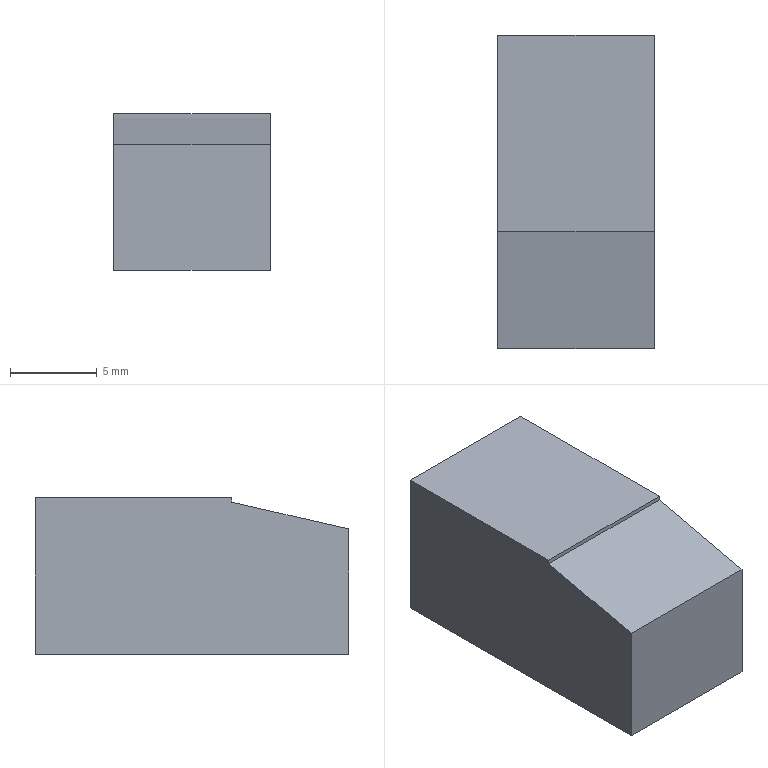Part | SolidWorks | features BaseBody 1 | 1 solid | 8 faces | box 9 x 18 x 9 mm | volume 1396 mm3 | plane 8
STEP:
#1=CARTESIAN_POINT('',(-102.,182.,178.223));
#2=VERTEX_POINT('',#1);
#3=CARTESIAN_POINT('',(-102.,188.726,179.763));
#4=VERTEX_POINT('',#3);
#5=CARTESIAN_POINT('',(-102.,199.493,182.228));
#6=DIRECTION('',(0.,0.9748,0.2232));
#7=VECTOR('',#6,1000.);
#8=LINE('',#5,#7);
#9=EDGE_CURVE('',#2,#4,#8,.T.);
#10=ORIENTED_EDGE('',*,*,#9,.T.);
#11=CARTESIAN_POINT('',(-102.,188.726,180.013));
#12=VERTEX_POINT('',#11);
#13=CARTESIAN_POINT('',(-102.,188.726,180.013));
#14=DIRECTION('',(0.,0.,1.));
#15=VECTOR('',#14,1000.);
#16=LINE('',#13,#15);
#17=EDGE_CURVE('',#4,#12,#16,.T.);
#18=ORIENTED_EDGE('',*,*,#17,.T.);
#19=CARTESIAN_POINT('',(-102.,200.,180.013));
#20=VERTEX_POINT('',#19);
#21=CARTESIAN_POINT('',(-102.,200.,180.013));
#22=DIRECTION('',(0.,-1.,0.));
#23=VECTOR('',#22,1000.);
#24=LINE('',#21,#23);
#25=EDGE_CURVE('',#20,#12,#24,.T.);
#26=ORIENTED_EDGE('',*,*,#25,.F.);
#27=CARTESIAN_POINT('',(-102.,200.,171.013));
#28=VERTEX_POINT('',#27);
#29=CARTESIAN_POINT('',(-102.,200.,180.013));
#30=DIRECTION('',(0.,0.,-1.));
#31=VECTOR('',#30,1000.);
#32=LINE('',#29,#31);
#33=EDGE_CURVE('',#20,#28,#32,.T.);
#34=ORIENTED_EDGE('',*,*,#33,.T.);
#35=CARTESIAN_POINT('',(-102.,182.,171.013));
#36=VERTEX_POINT('',#35);
#37=CARTESIAN_POINT('',(-102.,200.,171.013));
#38=DIRECTION('',(0.,-1.,0.));
#39=VECTOR('',#38,1000.);
#40=LINE('',#37,#39);
#41=EDGE_CURVE('',#28,#36,#40,.T.);
#42=ORIENTED_EDGE('',*,*,#41,.T.);
#43=CARTESIAN_POINT('',(-102.,182.,180.013));
#44=DIRECTION('',(0.,0.,-1.));
#45=VECTOR('',#44,1000.);
#46=LINE('',#43,#45);
#47=EDGE_CURVE('',#2,#36,#46,.T.);
#48=ORIENTED_EDGE('',*,*,#47,.F.);
#49=EDGE_LOOP('',(#10,#18,#26,#34,#42,#48));
#50=FACE_OUTER_BOUND('',#49,.T.);
#51=CARTESIAN_POINT('',(-102.,200.,180.013));
#52=DIRECTION('',(1.,0.,0.));
#53=DIRECTION('',(0.,0.,-1.));
#54=AXIS2_PLACEMENT_3D('',#51,#52,#53);
#55=PLANE('',#54);
#56=ADVANCED_FACE('',(#50),#55,.F.);
#57=CARTESIAN_POINT('',(-93.,182.,178.223));
#58=VERTEX_POINT('',#57);
#59=CARTESIAN_POINT('',(-93.,182.,171.013));
#60=VERTEX_POINT('',#59);
#61=CARTESIAN_POINT('',(-93.,182.,180.013));
#62=DIRECTION('',(0.,0.,-1.));
#63=VECTOR('',#62,1000.);
#64=LINE('',#61,#63);
#65=EDGE_CURVE('',#58,#60,#64,.T.);
#66=ORIENTED_EDGE('',*,*,#65,.F.);
#67=CARTESIAN_POINT('',(-71.07,182.,178.223));
#68=DIRECTION('',(-1.,0.,0.));
#69=VECTOR('',#68,1000.);
#70=LINE('',#67,#69);
#71=EDGE_CURVE('',#58,#2,#70,.T.);
#72=ORIENTED_EDGE('',*,*,#71,.T.);
#73=ORIENTED_EDGE('',*,*,#47,.T.);
#74=CARTESIAN_POINT('',(-102.,182.,171.013));
#75=DIRECTION('',(1.,0.,0.));
#76=VECTOR('',#75,1000.);
#77=LINE('',#74,#76);
#78=EDGE_CURVE('',#36,#60,#77,.T.);
#79=ORIENTED_EDGE('',*,*,#78,.T.);
#80=EDGE_LOOP('',(#66,#72,#73,#79));
#81=FACE_OUTER_BOUND('',#80,.T.);
#82=CARTESIAN_POINT('',(-102.,182.,180.013));
#83=DIRECTION('',(0.,1.,0.));
#84=DIRECTION('',(0.,0.,1.));
#85=AXIS2_PLACEMENT_3D('',#82,#83,#84);
#86=PLANE('',#85);
#87=ADVANCED_FACE('',(#81),#86,.F.);
#88=CARTESIAN_POINT('',(-93.,188.726,180.013));
#89=VERTEX_POINT('',#88);
#90=CARTESIAN_POINT('',(-93.,200.,180.013));
#91=VERTEX_POINT('',#90);
#92=CARTESIAN_POINT('',(-93.,188.,180.013));
#93=DIRECTION('',(0.,1.,0.));
#94=VECTOR('',#93,1000.);
#95=LINE('',#92,#94);
#96=EDGE_CURVE('',#89,#91,#95,.T.);
#97=ORIENTED_EDGE('',*,*,#96,.F.);
#98=CARTESIAN_POINT('',(-93.,188.726,179.763));
#99=VERTEX_POINT('',#98);
#100=CARTESIAN_POINT('',(-93.,188.726,180.013));
#101=DIRECTION('',(0.,0.,-1.));
#102=VECTOR('',#101,1000.);
#103=LINE('',#100,#102);
#104=EDGE_CURVE('',#89,#99,#103,.T.);
#105=ORIENTED_EDGE('',*,*,#104,.T.);
#106=CARTESIAN_POINT('',(-93.,188.091,179.618));
#107=DIRECTION('',(0.,-0.9748,-0.2232));
#108=VECTOR('',#107,1000.);
#109=LINE('',#106,#108);
#110=EDGE_CURVE('',#99,#58,#109,.T.);
#111=ORIENTED_EDGE('',*,*,#110,.T.);
#112=ORIENTED_EDGE('',*,*,#65,.T.);
#113=CARTESIAN_POINT('',(-93.,200.,171.013));
#114=VERTEX_POINT('',#113);
#115=CARTESIAN_POINT('',(-93.,188.,171.013));
#116=DIRECTION('',(0.,1.,0.));
#117=VECTOR('',#116,1000.);
#118=LINE('',#115,#117);
#119=EDGE_CURVE('',#60,#114,#118,.T.);
#120=ORIENTED_EDGE('',*,*,#119,.T.);
#121=CARTESIAN_POINT('',(-93.,200.,180.013));
#122=DIRECTION('',(0.,0.,-1.));
#123=VECTOR('',#122,1000.);
#124=LINE('',#121,#123);
#125=EDGE_CURVE('',#91,#114,#124,.T.);
#126=ORIENTED_EDGE('',*,*,#125,.F.);
#127=EDGE_LOOP('',(#97,#105,#111,#112,#120,#126));
#128=FACE_OUTER_BOUND('',#127,.T.);
#129=CARTESIAN_POINT('',(-93.,188.,180.013));
#130=DIRECTION('',(-1.,0.,0.));
#131=DIRECTION('',(0.,0.,1.));
#132=AXIS2_PLACEMENT_3D('',#129,#130,#131);
#133=PLANE('',#132);
#134=ADVANCED_FACE('',(#128),#133,.F.);
#135=CARTESIAN_POINT('',(-93.,200.,171.013));
#136=DIRECTION('',(-1.,0.,0.));
#137=VECTOR('',#136,1000.);
#138=LINE('',#135,#137);
#139=EDGE_CURVE('',#114,#28,#138,.T.);
#140=ORIENTED_EDGE('',*,*,#139,.T.);
#141=ORIENTED_EDGE('',*,*,#33,.F.);
#142=CARTESIAN_POINT('',(-93.,200.,180.013));
#143=DIRECTION('',(-1.,0.,0.));
#144=VECTOR('',#143,1000.);
#145=LINE('',#142,#144);
#146=EDGE_CURVE('',#91,#20,#145,.T.);
#147=ORIENTED_EDGE('',*,*,#146,.F.);
#148=ORIENTED_EDGE('',*,*,#125,.T.);
#149=EDGE_LOOP('',(#140,#141,#147,#148));
#150=FACE_OUTER_BOUND('',#149,.T.);
#151=CARTESIAN_POINT('',(-93.,200.,180.013));
#152=DIRECTION('',(0.,-1.,0.));
#153=DIRECTION('',(0.,0.,-1.));
#154=AXIS2_PLACEMENT_3D('',#151,#152,#153);
#155=PLANE('',#154);
#156=ADVANCED_FACE('',(#150),#155,.F.);
#157=CARTESIAN_POINT('',(-71.07,188.726,180.013));
#158=DIRECTION('',(-1.,0.,0.));
#159=VECTOR('',#158,1000.);
#160=LINE('',#157,#159);
#161=EDGE_CURVE('',#89,#12,#160,.T.);
#162=ORIENTED_EDGE('',*,*,#161,.F.);
#163=ORIENTED_EDGE('',*,*,#96,.T.);
#164=ORIENTED_EDGE('',*,*,#146,.T.);
#165=ORIENTED_EDGE('',*,*,#25,.T.);
#166=EDGE_LOOP('',(#162,#163,#164,#165));
#167=FACE_OUTER_BOUND('',#166,.T.);
#168=CARTESIAN_POINT('',(7.,0.,180.013));
#169=DIRECTION('',(0.,0.,1.));
#170=DIRECTION('',(1.,0.,0.));
#171=AXIS2_PLACEMENT_3D('',#168,#169,#170);
#172=PLANE('',#171);
#173=ADVANCED_FACE('',(#167),#172,.T.);
#174=ORIENTED_EDGE('',*,*,#41,.F.);
#175=ORIENTED_EDGE('',*,*,#139,.F.);
#176=ORIENTED_EDGE('',*,*,#119,.F.);
#177=ORIENTED_EDGE('',*,*,#78,.F.);
#178=EDGE_LOOP('',(#174,#175,#176,#177));
#179=FACE_OUTER_BOUND('',#178,.T.);
#180=CARTESIAN_POINT('',(7.,0.,171.013));
#181=DIRECTION('',(0.,0.,1.));
#182=DIRECTION('',(1.,0.,0.));
#183=AXIS2_PLACEMENT_3D('',#180,#181,#182);
#184=PLANE('',#183);
#185=ADVANCED_FACE('',(#179),#184,.F.);
#186=ORIENTED_EDGE('',*,*,#71,.F.);
#187=ORIENTED_EDGE('',*,*,#110,.F.);
#188=CARTESIAN_POINT('',(-71.07,188.726,179.763));
#189=DIRECTION('',(1.,0.,0.));
#190=VECTOR('',#189,1000.);
#191=LINE('',#188,#190);
#192=EDGE_CURVE('',#4,#99,#191,.T.);
#193=ORIENTED_EDGE('',*,*,#192,.F.);
#194=ORIENTED_EDGE('',*,*,#9,.F.);
#195=EDGE_LOOP('',(#186,#187,#193,#194));
#196=FACE_OUTER_BOUND('',#195,.T.);
#197=CARTESIAN_POINT('',(-71.07,188.726,179.763));
#198=DIRECTION('',(0.,0.2232,-0.9748));
#199=DIRECTION('',(0.,-0.9748,-0.2232));
#200=AXIS2_PLACEMENT_3D('',#197,#198,#199);
#201=PLANE('',#200);
#202=ADVANCED_FACE('',(#196),#201,.F.);
#203=ORIENTED_EDGE('',*,*,#192,.T.);
#204=ORIENTED_EDGE('',*,*,#104,.F.);
#205=ORIENTED_EDGE('',*,*,#161,.T.);
#206=ORIENTED_EDGE('',*,*,#17,.F.);
#207=EDGE_LOOP('',(#203,#204,#205,#206));
#208=FACE_OUTER_BOUND('',#207,.T.);
#209=CARTESIAN_POINT('',(-71.07,188.726,180.013));
#210=DIRECTION('',(0.,1.,0.));
#211=DIRECTION('',(0.,0.,-1.));
#212=AXIS2_PLACEMENT_3D('',#209,#210,#211);
#213=PLANE('',#212);
#214=ADVANCED_FACE('',(#208),#213,.F.);
#215=CLOSED_SHELL('',(#56,#87,#134,#156,#173,#185,#202,#214));
#216=MANIFOLD_SOLID_BREP('',#215);
#217=CARTESIAN_POINT('',(0.,0.,0.));
#218=DIRECTION('',(0.,0.,1.));
#219=DIRECTION('',(1.,0.,0.));
#220=AXIS2_PLACEMENT_3D('',#217,#218,#219);
#221=(LENGTH_UNIT()NAMED_UNIT(*)SI_UNIT(.MILLI.,.METRE.));
#222=UNCERTAINTY_MEASURE_WITH_UNIT(LENGTH_MEASURE(0.00001),#221,'','');
#223=(NAMED_UNIT(*)PLANE_ANGLE_UNIT()SI_UNIT($,.RADIAN.));
#224=(NAMED_UNIT(*)SI_UNIT($,.STERADIAN.)SOLID_ANGLE_UNIT());
#225=(GEOMETRIC_REPRESENTATION_CONTEXT(3)GLOBAL_UNCERTAINTY_ASSIGNED_CONTEXT((#222))GLOBAL_UNIT_ASSIGNED_CONTEXT((#221,#223,#224))REPRESENTATION_CONTEXT('',''));
#226=ADVANCED_BREP_SHAPE_REPRESENTATION('',(#216,#220),#225);